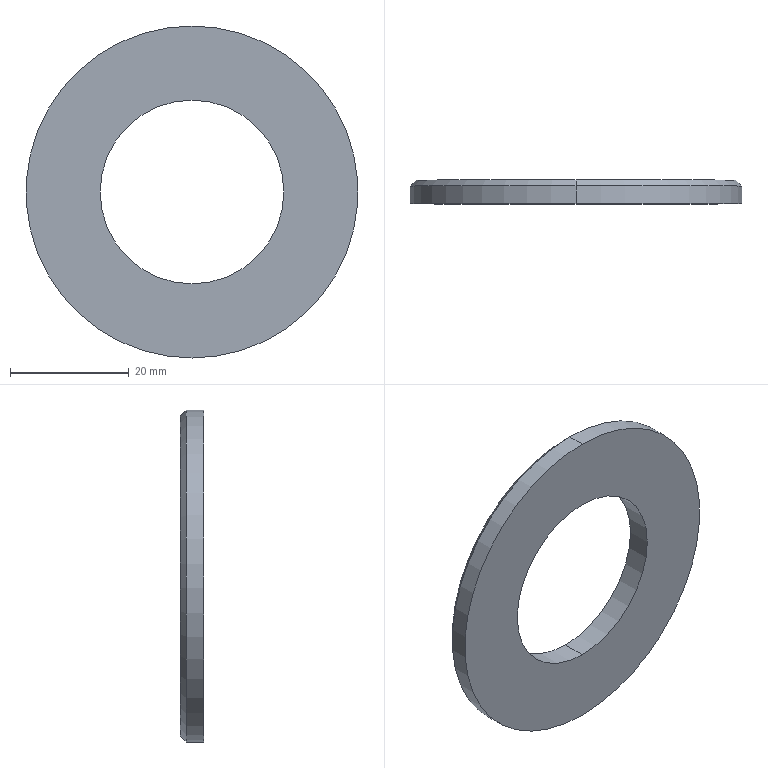Part | SolidWorks | features Revolution 1 | 1 solid | 8 faces | box 56 x 4 x 56 mm | volume 6746 mm3 | cylinder 4 | cone 2 | plane 2 | commonest cylinder face diameters 31 x2 56 x2
STEP:
#1=CARTESIAN_POINT('',(0.,11.645,-28.));
#2=VERTEX_POINT('',#1);
#3=CARTESIAN_POINT('',(0.,11.645,28.));
#4=VERTEX_POINT('',#3);
#5=CARTESIAN_POINT('',(0.,11.645,0.));
#6=DIRECTION('',(0.,-1.,0.));
#7=DIRECTION('',(0.,0.,-1.));
#8=AXIS2_PLACEMENT_3D('',#5,#6,#7);
#9=CIRCLE('',#8,28.);
#10=EDGE_CURVE('',#2,#4,#9,.T.);
#11=ORIENTED_EDGE('',*,*,#10,.T.);
#12=CARTESIAN_POINT('',(0.,8.645,28.));
#13=VERTEX_POINT('',#12);
#14=CARTESIAN_POINT('',(0.,0.,28.));
#15=DIRECTION('',(0.,-1.,0.));
#16=VECTOR('',#15,1000.);
#17=LINE('',#14,#16);
#18=EDGE_CURVE('',#4,#13,#17,.T.);
#19=ORIENTED_EDGE('',*,*,#18,.T.);
#20=CARTESIAN_POINT('',(0.,8.645,-28.));
#21=VERTEX_POINT('',#20);
#22=CARTESIAN_POINT('',(0.,8.645,0.));
#23=DIRECTION('',(0.,-1.,0.));
#24=DIRECTION('',(0.,0.,-1.));
#25=AXIS2_PLACEMENT_3D('',#22,#23,#24);
#26=CIRCLE('',#25,28.);
#27=EDGE_CURVE('',#21,#13,#26,.T.);
#28=ORIENTED_EDGE('',*,*,#27,.F.);
#29=CARTESIAN_POINT('',(0.,0.,-28.));
#30=DIRECTION('',(0.,-1.,0.));
#31=VECTOR('',#30,1000.);
#32=LINE('',#29,#31);
#33=EDGE_CURVE('',#2,#21,#32,.T.);
#34=ORIENTED_EDGE('',*,*,#33,.F.);
#35=EDGE_LOOP('',(#11,#19,#28,#34));
#36=FACE_OUTER_BOUND('',#35,.T.);
#37=CARTESIAN_POINT('',(0.,0.,0.));
#38=DIRECTION('',(0.,-1.,0.));
#39=DIRECTION('',(0.,0.,-1.));
#40=AXIS2_PLACEMENT_3D('',#37,#38,#39);
#41=CYLINDRICAL_SURFACE('',#40,28.);
#42=ADVANCED_FACE('',(#36),#41,.T.);
#43=CARTESIAN_POINT('',(0.,12.645,-27.));
#44=VERTEX_POINT('',#43);
#45=CARTESIAN_POINT('',(0.,12.645,27.));
#46=VERTEX_POINT('',#45);
#47=CARTESIAN_POINT('',(0.,12.645,0.));
#48=DIRECTION('',(0.,-1.,0.));
#49=DIRECTION('',(0.,0.,-1.));
#50=AXIS2_PLACEMENT_3D('',#47,#48,#49);
#51=CIRCLE('',#50,27.);
#52=EDGE_CURVE('',#44,#46,#51,.T.);
#53=ORIENTED_EDGE('',*,*,#52,.T.);
#54=CARTESIAN_POINT('',(0.,12.645,27.));
#55=DIRECTION('',(0.,-0.7071,0.7071));
#56=VECTOR('',#55,1000.);
#57=LINE('',#54,#56);
#58=EDGE_CURVE('',#46,#4,#57,.T.);
#59=ORIENTED_EDGE('',*,*,#58,.T.);
#60=ORIENTED_EDGE('',*,*,#10,.F.);
#61=CARTESIAN_POINT('',(0.,12.645,-27.));
#62=DIRECTION('',(0.,-0.7071,-0.7071));
#63=VECTOR('',#62,1000.);
#64=LINE('',#61,#63);
#65=EDGE_CURVE('',#44,#2,#64,.T.);
#66=ORIENTED_EDGE('',*,*,#65,.F.);
#67=EDGE_LOOP('',(#53,#59,#60,#66));
#68=FACE_OUTER_BOUND('',#67,.T.);
#69=CARTESIAN_POINT('',(0.,12.645,0.));
#70=DIRECTION('',(0.,-1.,0.));
#71=DIRECTION('',(0.,0.,-1.));
#72=AXIS2_PLACEMENT_3D('',#69,#70,#71);
#73=CONICAL_SURFACE('',#72,27.,0.7854);
#74=ADVANCED_FACE('',(#68),#73,.T.);
#75=CARTESIAN_POINT('',(0.,12.645,15.5));
#76=VERTEX_POINT('',#75);
#77=CARTESIAN_POINT('',(0.,12.645,-15.5));
#78=VERTEX_POINT('',#77);
#79=CARTESIAN_POINT('',(0.,12.645,0.));
#80=DIRECTION('',(0.,-1.,0.));
#81=DIRECTION('',(0.,0.,-1.));
#82=AXIS2_PLACEMENT_3D('',#79,#80,#81);
#83=CIRCLE('',#82,15.5);
#84=EDGE_CURVE('',#76,#78,#83,.T.);
#85=ORIENTED_EDGE('',*,*,#84,.F.);
#86=CARTESIAN_POINT('',(0.,8.645,15.5));
#87=VERTEX_POINT('',#86);
#88=CARTESIAN_POINT('',(0.,0.,15.5));
#89=DIRECTION('',(0.,-1.,0.));
#90=VECTOR('',#89,1000.);
#91=LINE('',#88,#90);
#92=EDGE_CURVE('',#76,#87,#91,.T.);
#93=ORIENTED_EDGE('',*,*,#92,.T.);
#94=CARTESIAN_POINT('',(0.,8.645,-15.5));
#95=VERTEX_POINT('',#94);
#96=CARTESIAN_POINT('',(0.,8.645,0.));
#97=DIRECTION('',(0.,-1.,0.));
#98=DIRECTION('',(0.,0.,-1.));
#99=AXIS2_PLACEMENT_3D('',#96,#97,#98);
#100=CIRCLE('',#99,15.5);
#101=EDGE_CURVE('',#87,#95,#100,.T.);
#102=ORIENTED_EDGE('',*,*,#101,.T.);
#103=CARTESIAN_POINT('',(0.,0.,-15.5));
#104=DIRECTION('',(0.,-1.,0.));
#105=VECTOR('',#104,1000.);
#106=LINE('',#103,#105);
#107=EDGE_CURVE('',#78,#95,#106,.T.);
#108=ORIENTED_EDGE('',*,*,#107,.F.);
#109=EDGE_LOOP('',(#85,#93,#102,#108));
#110=FACE_OUTER_BOUND('',#109,.T.);
#111=CARTESIAN_POINT('',(0.,0.,0.));
#112=DIRECTION('',(0.,-1.,0.));
#113=DIRECTION('',(0.,0.,-1.));
#114=AXIS2_PLACEMENT_3D('',#111,#112,#113);
#115=CYLINDRICAL_SURFACE('',#114,15.5);
#116=ADVANCED_FACE('',(#110),#115,.F.);
#117=ORIENTED_EDGE('',*,*,#92,.F.);
#118=CARTESIAN_POINT('',(0.,12.645,0.));
#119=DIRECTION('',(0.,-1.,0.));
#120=DIRECTION('',(0.,0.,-1.));
#121=AXIS2_PLACEMENT_3D('',#118,#119,#120);
#122=CIRCLE('',#121,15.5);
#123=EDGE_CURVE('',#78,#76,#122,.T.);
#124=ORIENTED_EDGE('',*,*,#123,.F.);
#125=ORIENTED_EDGE('',*,*,#107,.T.);
#126=CARTESIAN_POINT('',(0.,8.645,0.));
#127=DIRECTION('',(0.,-1.,0.));
#128=DIRECTION('',(0.,0.,-1.));
#129=AXIS2_PLACEMENT_3D('',#126,#127,#128);
#130=CIRCLE('',#129,15.5);
#131=EDGE_CURVE('',#95,#87,#130,.T.);
#132=ORIENTED_EDGE('',*,*,#131,.T.);
#133=EDGE_LOOP('',(#117,#124,#125,#132));
#134=FACE_OUTER_BOUND('',#133,.T.);
#135=CARTESIAN_POINT('',(0.,0.,0.));
#136=DIRECTION('',(0.,-1.,0.));
#137=DIRECTION('',(0.,0.,-1.));
#138=AXIS2_PLACEMENT_3D('',#135,#136,#137);
#139=CYLINDRICAL_SURFACE('',#138,15.5);
#140=ADVANCED_FACE('',(#134),#139,.F.);
#141=ORIENTED_EDGE('',*,*,#52,.F.);
#142=CARTESIAN_POINT('',(0.,12.645,0.));
#143=DIRECTION('',(0.,-1.,0.));
#144=DIRECTION('',(0.,0.,-1.));
#145=AXIS2_PLACEMENT_3D('',#142,#143,#144);
#146=CIRCLE('',#145,27.);
#147=EDGE_CURVE('',#46,#44,#146,.T.);
#148=ORIENTED_EDGE('',*,*,#147,.F.);
#149=EDGE_LOOP('',(#141,#148));
#150=FACE_OUTER_BOUND('',#149,.T.);
#151=ORIENTED_EDGE('',*,*,#123,.T.);
#152=ORIENTED_EDGE('',*,*,#84,.T.);
#153=EDGE_LOOP('',(#151,#152));
#154=FACE_BOUND('',#153,.T.);
#155=CARTESIAN_POINT('',(-15.5,12.645,0.));
#156=DIRECTION('',(0.,-1.,0.));
#157=DIRECTION('',(0.,0.,-1.));
#158=AXIS2_PLACEMENT_3D('',#155,#156,#157);
#159=PLANE('',#158);
#160=ADVANCED_FACE('',(#150,#154),#159,.F.);
#161=ORIENTED_EDGE('',*,*,#58,.F.);
#162=ORIENTED_EDGE('',*,*,#147,.T.);
#163=ORIENTED_EDGE('',*,*,#65,.T.);
#164=CARTESIAN_POINT('',(0.,11.645,0.));
#165=DIRECTION('',(0.,-1.,0.));
#166=DIRECTION('',(0.,0.,-1.));
#167=AXIS2_PLACEMENT_3D('',#164,#165,#166);
#168=CIRCLE('',#167,28.);
#169=EDGE_CURVE('',#4,#2,#168,.T.);
#170=ORIENTED_EDGE('',*,*,#169,.F.);
#171=EDGE_LOOP('',(#161,#162,#163,#170));
#172=FACE_OUTER_BOUND('',#171,.T.);
#173=CARTESIAN_POINT('',(0.,12.645,0.));
#174=DIRECTION('',(0.,-1.,0.));
#175=DIRECTION('',(0.,0.,-1.));
#176=AXIS2_PLACEMENT_3D('',#173,#174,#175);
#177=CONICAL_SURFACE('',#176,27.,0.7854);
#178=ADVANCED_FACE('',(#172),#177,.T.);
#179=ORIENTED_EDGE('',*,*,#18,.F.);
#180=ORIENTED_EDGE('',*,*,#169,.T.);
#181=ORIENTED_EDGE('',*,*,#33,.T.);
#182=CARTESIAN_POINT('',(0.,8.645,0.));
#183=DIRECTION('',(0.,-1.,0.));
#184=DIRECTION('',(0.,0.,-1.));
#185=AXIS2_PLACEMENT_3D('',#182,#183,#184);
#186=CIRCLE('',#185,28.);
#187=EDGE_CURVE('',#13,#21,#186,.T.);
#188=ORIENTED_EDGE('',*,*,#187,.F.);
#189=EDGE_LOOP('',(#179,#180,#181,#188));
#190=FACE_OUTER_BOUND('',#189,.T.);
#191=CARTESIAN_POINT('',(0.,0.,0.));
#192=DIRECTION('',(0.,-1.,0.));
#193=DIRECTION('',(0.,0.,-1.));
#194=AXIS2_PLACEMENT_3D('',#191,#192,#193);
#195=CYLINDRICAL_SURFACE('',#194,28.);
#196=ADVANCED_FACE('',(#190),#195,.T.);
#197=ORIENTED_EDGE('',*,*,#131,.F.);
#198=ORIENTED_EDGE('',*,*,#101,.F.);
#199=EDGE_LOOP('',(#197,#198));
#200=FACE_BOUND('',#199,.T.);
#201=ORIENTED_EDGE('',*,*,#27,.T.);
#202=ORIENTED_EDGE('',*,*,#187,.T.);
#203=EDGE_LOOP('',(#201,#202));
#204=FACE_OUTER_BOUND('',#203,.T.);
#205=CARTESIAN_POINT('',(-15.5,8.645,0.));
#206=DIRECTION('',(0.,1.,0.));
#207=DIRECTION('',(0.,0.,1.));
#208=AXIS2_PLACEMENT_3D('',#205,#206,#207);
#209=PLANE('',#208);
#210=ADVANCED_FACE('',(#200,#204),#209,.F.);
#211=CLOSED_SHELL('',(#42,#74,#116,#140,#160,#178,#196,#210));
#212=MANIFOLD_SOLID_BREP('',#211);
#213=CARTESIAN_POINT('',(0.,0.,0.));
#214=DIRECTION('',(0.,0.,1.));
#215=DIRECTION('',(1.,0.,0.));
#216=AXIS2_PLACEMENT_3D('',#213,#214,#215);
#217=(LENGTH_UNIT()NAMED_UNIT(*)SI_UNIT(.MILLI.,.METRE.));
#218=UNCERTAINTY_MEASURE_WITH_UNIT(LENGTH_MEASURE(0.00001),#217,'','');
#219=(NAMED_UNIT(*)PLANE_ANGLE_UNIT()SI_UNIT($,.RADIAN.));
#220=(NAMED_UNIT(*)SI_UNIT($,.STERADIAN.)SOLID_ANGLE_UNIT());
#221=(GEOMETRIC_REPRESENTATION_CONTEXT(3)GLOBAL_UNCERTAINTY_ASSIGNED_CONTEXT((#218))GLOBAL_UNIT_ASSIGNED_CONTEXT((#217,#219,#220))REPRESENTATION_CONTEXT('',''));
#222=ADVANCED_BREP_SHAPE_REPRESENTATION('',(#212,#216),#221);